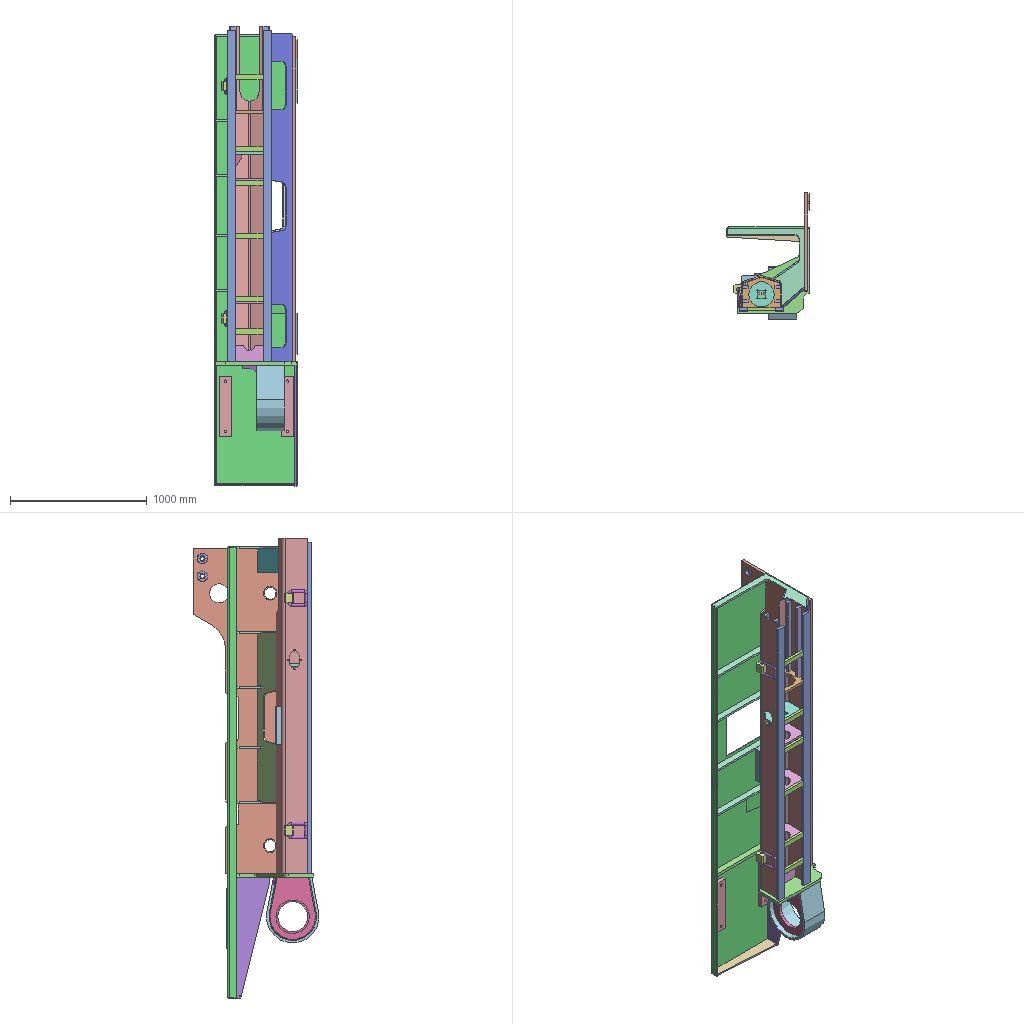Assembly | SolidWorks | 36 different items | 56 placed | box 605 x 919 x 3365 mm
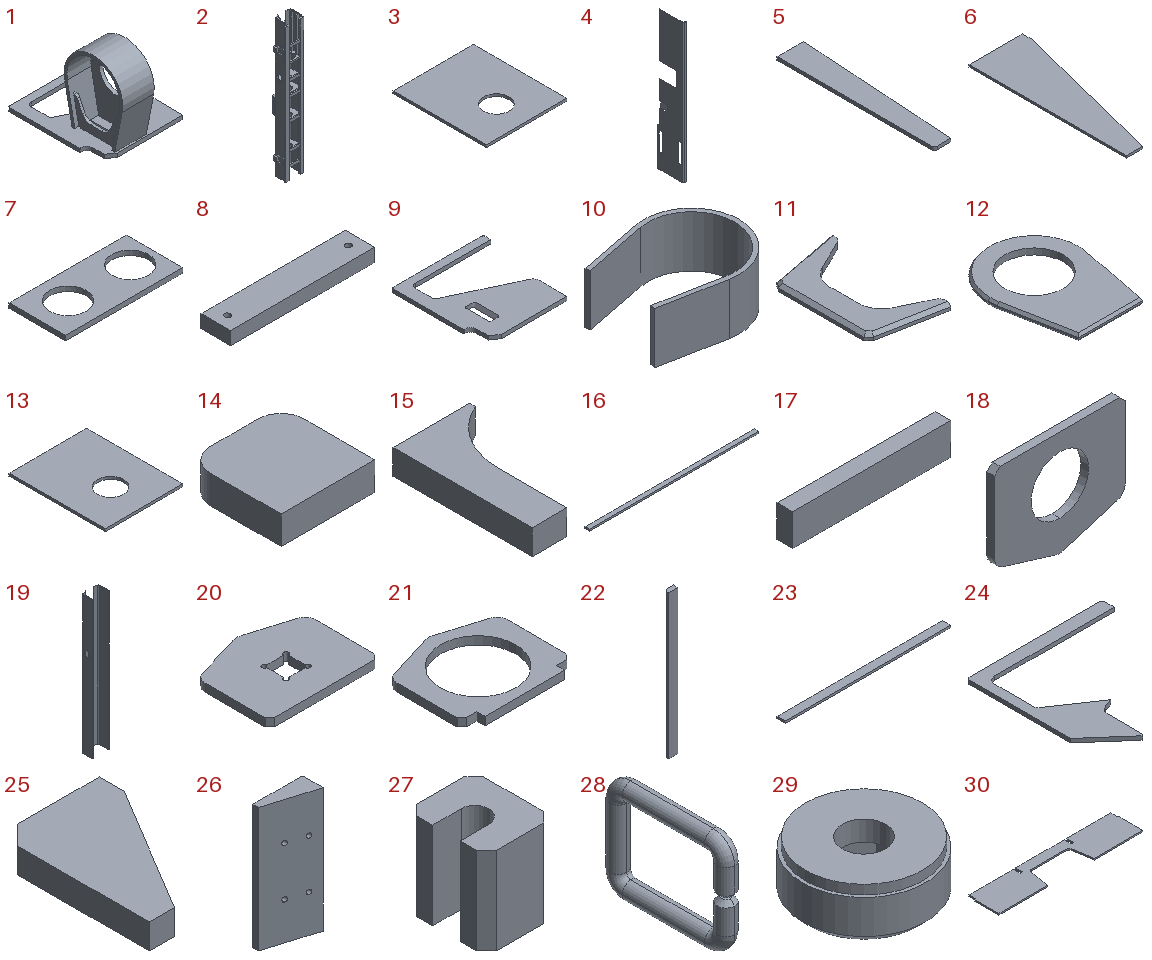Parts list (item | name | quantity | parent item | size | volume | features):
1 | (subassembly) | x1 | - | 600 x 663.219 x 507.5 mm | 12024665 mm3 | -
2 | (subassembly) | x1 | - | 364.5 x 260.017 x 2455 mm | 31232194 mm3 | features LocalLPattern 11, ReferencePattern 11, MateUpdatePoint 2
3 | - | x1 | - | 320 x 370 x 10 mm | 1105460 mm3 | features Extrusion 1
4 | - | x1 | - | 65 x 605 x 3295 mm | 14782369 mm3 | features ICE 2, Extrusion 1, NetBlend 1
5 | - | x1 | - | 96 x 578 x 12 mm | 542484 mm3 | features Extrusion 1
6 | - | x1 | - | 300 x 885 x 12 mm | 2143920 mm3 | features Extrusion 1
7 | - | x1 | - | 245 x 118 x 10 mm | 198371 mm3 | features Extrusion 1
8 | - | x2 | - | 440 x 90 x 40 mm | 1564758 mm3 | features Extrusion 1, HoleWzd 1
9 | - | x1 | in 1 | 600 x 622.5 x 25 mm | 4943914 mm3 | features BlendCut 1, Extrusion 1
10 | - | x1 | in 1 | 482.5 x 385 x 207.5 mm | 4343346 mm3 | features Extrusion 1
11 | - | x1 | in 1 | 180 x 311.6 x 16 mm | 387961 mm3 | features Chamfer 2, Extrusion 1
12 | - | x1 | in 1 | 347 x 463.5 x 25 mm | 2272890 mm3 | features Chamfer 2, Extrusion 1, ICE 1
13 | - | x1 | - | 300 x 370 x 10 mm | 1031460 mm3 | features Extrusion 1
14 | - | x1 | in 1 | 40 x 40 x 12 mm | 18685 mm3 | features Extrusion 1
15 | - | x1 | in 1 | 55 x 100 x 18 mm | 54165 mm3 | features Extrusion 1
16 | - | x2 | in 2 | 2425 x 63 x 25 mm | 3819375 mm3 | features Extrusion 1
17 | - | x6 | in 2 | 199 x 20 x 40 mm | 159200 mm3 | features Extrusion 1
18 | - | x3 | in 2 | 273 x 16 x 219.3 mm | 688093 mm3 | features Extrusion 1
19 | - | x1 | in 2 | 295 x 232 x 2455 mm | 15250128 mm3 | features ICE 2, Extrusion 1, HoleWzd 1
20 | - | x1 | in 2 | 273 x 219.3 x 20 mm | 1021205 mm3 | features Extrusion 1
21 | - | x1 | in 2 | 273 x 239.5 x 20 mm | 622595 mm3 | features Extrusion 1
22 | - | x4 | in 2 | 39 x 20 x 620 mm | 463760 mm3 | features Chamfer 1, Extrusion 1
23 | - | x1 | in 2 | 620 x 30 x 8 mm | 148800 mm3 | features Extrusion 1
24 | - | x5 | - | 560 x 566.399 x 16 mm | 1167723 mm3 | features Extrusion 1
25 | - | x1 | in 2 | 80 x 120 x 20 mm | 129750 mm3 | features Extrusion 1
26 | - | x1 | in 2 | 112 x 46.7 x 280 mm | 914034 mm3 | features Extrusion 1, HoleWzd 1
27 | - | x2 | in 2 | 54 x 64 x 70 mm | 184235 mm3 | features Extrusion 1
28 | - | x2 | in 2 | 20 x 146 x 120 mm | 131972 mm3 | features Chamfer 1, Sweep 1
29 | - | x2 | - | 80 x 80 x 33 mm | 125576 mm3 | features ICE 3, Chamfer 1, Extrusion 1
30 | - | x1 | - | 1240 x 268 x 12 mm | 3104432 mm3 | features Extrusion 1
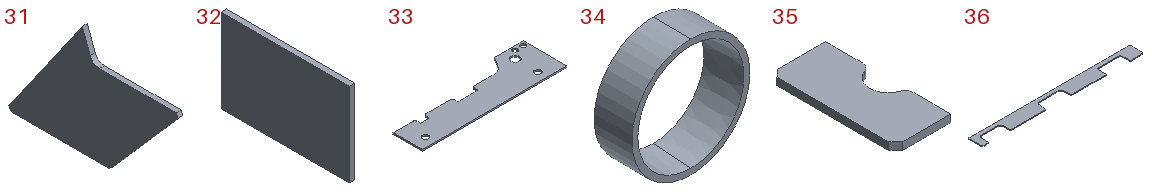31 | - | x1 | - | 10 x 341.699 x 222 mm | 386732 mm3 | features Extrusion 1
32 | - | x1 | - | 12 x 268 x 175 mm | 562800 mm3 | features Extrusion 1
33 | - | x1 | - | 2375 x 714.5 x 25 mm | 29470631 mm3 | features Extrusion 1
34 | - | x2 | - | 100 x 32 x 100 mm | 56666 mm3 | features Revolution 1
35 | - | x1 | - | 120 x 273 x 16 mm | 478824 mm3 | features Extrusion 1
36 | - | x1 | - | 2400 x 207 x 12 mm | 4150722 mm3 | features Extrusion 1
Mates (type | each side: item.copy, entity, surface, feature):
In the top assembly
Coincident | 19.1 face plane Boss-Extrude1 | 24.1 face plane Boss-Extrude1
DistanceDim | 24.1 face plane Boss-Extrude1 | 33.1 face plane Boss-Extrude1
DistanceDim | 33.1 face plane Boss-Extrude1 | 16.1 face plane Boss-Extrude1
Coincident | 24.2 face plane Boss-Extrude1 | 36.1 face plane Boss-Extrude1
Coincident | 33.1 face plane Boss-Extrude1 | 36.1 edge
Coincident | 24.2 face plane Boss-Extrude1 | 30.1 face plane Boss-Extrude1
DistanceDim | 30.1 face plane Boss-Extrude1 | 24.1 face plane Boss-Extrude1
Coincident | 33.1 face plane Boss-Extrude1 | 30.1 edge
DistanceDim | 31.1 face plane Boss-Extrude1 | 19.1 face plane Boss-Extrude1
Coincident | 19.1 face plane Boss-Extrude1 | 31.1 face plane Boss-Extrude1
Coincident | 24.3 edge | 31.1 face plane Boss-Extrude1
Coincident | 33.1 face plane Boss-Extrude1 | 24.4 face plane Boss-Extrude1 | 2 times
Coincident | 24.3 face plane Boss-Extrude1 | 24.4 face plane Boss-Extrude1
Coincident | 24.4 face plane Boss-Extrude1 | 32.1 face plane Boss-Extrude1 | 2 times
Coincident | 33.1 face plane Boss-Extrude1 | 32.1 edge
Coincident | 33.1 face plane Boss-Extrude1 | 4.1 face plane Cut-Extrude1 | 2 times
DistanceDim | 8.1 face plane Boss-Extrude1 | 4.1 face plane Boss-Extrude1
Coincident | 4.1 face plane Cut-Extrude1 | 8.1 face plane Boss-Extrude1 | 2 times
DistanceDim | 8.2 face plane Boss-Extrude1 | 4.1 face plane Boss-Extrude1
Coincident | 4.1 face plane Cut-Extrude1 | 8.2 face plane Boss-Extrude1 | 2 times
DistanceDim | 6.1 face plane Boss-Extrude1 | 4.1 face plane Boss-Extrude1
Coincident | 6.1 face plane Boss-Extrude1 | 4.1 face plane Boss-Extrude1
Coincident | 5.1 face plane Boss-Extrude1 | 6.1 face plane Boss-Extrude1
Coincident | 5.1 face plane Boss-Extrude1 | 4.1 face plane Boss-Extrude1
DistanceDim | 5.1 face plane Boss-Extrude1 | 6.1 face plane Boss-Extrude1
Concentric | 33.1 face cylinder Boss-Extrude1 | 13.1 face cylinder Boss-Extrude1
Coincident | 33.1 face plane Boss-Extrude1 | 13.1 face plane Boss-Extrude1
Concentric | 33.1 face cylinder Boss-Extrude1 | 34.1 face cylinder Revolve1
Coincident | 13.1 face plane Boss-Extrude1 | 34.1 face plane Revolve1
Concentric | 33.1 face cylinder Boss-Extrude1 | 34.2 face cylinder Revolve1
Coincident | 19.1 face plane Boss-Extrude1 | 35.1 face plane Boss-Extrude1
DistanceDim | 35.1 face plane Boss-Extrude1 | 16.2 face plane Boss-Extrude1
Concentric | 33.1 face cylinder Boss-Extrude1 | 3.1 face cylinder Boss-Extrude1
Coincident | 33.1 face plane Boss-Extrude1 | 3.1 face plane Boss-Extrude1
Parallel | 33.1 face plane Boss-Extrude1 | 3.1 face plane Boss-Extrude1
Coincident | 34.2 face plane Revolve1 | 3.1 face plane Boss-Extrude1
Concentric | 33.1 face cylinder Boss-Extrude1 | 7.1 face cylinder Boss-Extrude1 | 2 times
Coincident | 33.1 face plane Boss-Extrude1 | 7.1 face plane Boss-Extrude1
Concentric | 33.1 face cylinder Boss-Extrude1 | 29.1 face cylinder Boss-Extrude1
Concentric | 33.1 face cylinder Boss-Extrude1 | 29.2 face cylinder Boss-Extrude1
Coincident | 7.1 face plane Boss-Extrude1 | 29.2 face plane Cut-Extrude1
Coincident | 7.1 face plane Boss-Extrude1 | 29.1 face plane Cut-Extrude1
Coincident | 4.1 face plane Boss-Extrude1 | 9.1 face plane Boss-Extrude1
Coincident | 16.2 face plane Boss-Extrude1 | 9.1 face plane Boss-Extrude1
DistanceDim | 9.1 face plane Boss-Extrude1 | 16.2 face plane Boss-Extrude1
DistanceDim | 9.1 face plane Boss-Extrude1 | 33.1 face plane Boss-Extrude1
In subassembly 1
Coincident | 9.2 face plane Boss-Extrude1 | 12.1 face plane Boss-Extrude1
DistanceDim | 12.1 face plane Boss-Extrude1 | 9.2 face plane Boss-Extrude1
Concentric | 12.1 face cylinder Boss-Extrude1 | 10.1 face cylinder Boss-Extrude1
DistanceDim | 12.1 face plane Boss-Extrude1 | 10.1 face plane Boss-Extrude1
Parallel | 12.1 face plane Boss-Extrude1 | 10.1 face plane Boss-Extrude1
DistanceDim | 10.1 face plane Boss-Extrude1 | 11.1 face plane Boss-Extrude1
Coincident | 9.2 face plane Boss-Extrude1 | 11.1 face plane Boss-Extrude1
Coincident | 10.1 face plane Boss-Extrude1 | 11.1 edge
Coincident | 10.1 face plane Boss-Extrude1 | 15.1 face plane Boss-Extrude1 | 2 times
Coincident | 9.2 face plane Boss-Extrude1 | 15.1 edge
Tangent | 10.1 face cylinder Boss-Extrude1 | 14.1 face plane Boss-Extrude1
DistanceDim | 14.1 face plane Boss-Extrude1 | 9.2 face plane Boss-Extrude1
DistanceDim | 14.1 face plane Boss-Extrude1 | 10.1 face plane Boss-Extrude1
DistanceDim | 10.1 edge | 9.2 face plane Boss-Extrude1
In subassembly 2
DistanceDim | 16.3 face plane Boss-Extrude1 | 19.2 face plane Boss-Extrude1
Coincident | 19.2 face plane Boss-Extrude1 | 16.3 face plane Boss-Extrude1 | 2 times
Coincident | 19.2 face plane Boss-Extrude1 | 16.4 face plane Boss-Extrude1 | 2 times
DistanceDim | 16.4 face plane Boss-Extrude1 | 19.2 face plane Boss-Extrude1
Coincident | 16.4 face plane Boss-Extrude1 | 17.1 face plane Boss-Extrude1 | 2 times
DistanceDim | 17.1 face plane Boss-Extrude1 | 16.4 face plane Boss-Extrude1
Coincident | 16.4 face plane Boss-Extrude1 | 18.1 face plane Boss-Extrude1
DistanceDim | 18.1 face plane Boss-Extrude1 | 19.2 face plane Boss-Extrude1 | 2 times
DistanceDim | 20.1 face plane Boss-Extrude1 | 18.2 face plane Boss-Extrude1
Coincident | 16.3 face plane Boss-Extrude1 | 20.1 face plane Boss-Extrude1
DistanceDim | 19.2 face plane Boss-Extrude1 | 20.1 face plane Boss-Extrude1
DistanceDim | 21.1 face plane Boss-Extrude1 | 20.1 face plane Boss-Extrude1
Coincident | 16.4 face plane Boss-Extrude1 | 21.1 face plane Boss-Extrude1
DistanceDim | 21.1 face plane Boss-Extrude1 | 19.2 face plane Boss-Extrude1
Coincident | 19.2 face plane Boss-Extrude1 | 22.1 face plane Boss-Extrude1
Coincident | 21.1 face plane Boss-Extrude1 | 22.1 face plane Boss-Extrude1
DistanceDim | 22.1 face plane Boss-Extrude1 | 16.4 face plane Boss-Extrude1
Coincident | 19.2 face plane Boss-Extrude1 | 22.2 face plane Boss-Extrude1
DistanceDim | 22.2 face plane Boss-Extrude1 | 16.3 face plane Boss-Extrude1
Coincident | 21.1 face plane Boss-Extrude1 | 22.2 face plane Boss-Extrude1
DistanceDim | 23.1 face plane Boss-Extrude1 | 22.3 face plane Boss-Extrude1
Coincident | 22.3 face plane Boss-Extrude1 | 23.1 face plane Boss-Extrude1
Coincident | 21.1 face plane Boss-Extrude1 | 23.1 face plane Boss-Extrude1
Coincident | 20.1 face plane Boss-Extrude1 | 25.1 face plane Boss-Extrude1
Coincident | 19.2 face plane Boss-Extrude1 | 25.1 face plane Boss-Extrude1
DistanceDim | 25.1 face plane Boss-Extrude1 | 16.4 face plane Boss-Extrude1
Concentric | 27.1 face cylinder Boss-Extrude1 | 28.1 face cylinder Sweep1
DistanceDim | 27.1 face plane Boss-Extrude1 | 16.3 face plane Boss-Extrude1
DistanceDim | 27.1 face plane Boss-Extrude1 | 28.1 face cylinder Sweep1
Coincident | 19.2 face plane Boss-Extrude1 | 27.1 face plane Boss-Extrude1
DistanceDim | 27.1 face plane Boss-Extrude1 | 16.4 face plane Boss-Extrude1
Coincident | 19.2 face plane Boss-Extrude1 | 26.1 face plane Boss-Extrude1
Coincident | 19.2 face plane Boss-Extrude1 | 26.1 edge
DistanceDim | 26.1 face plane Boss-Extrude1 | 16.4 face plane Boss-Extrude1